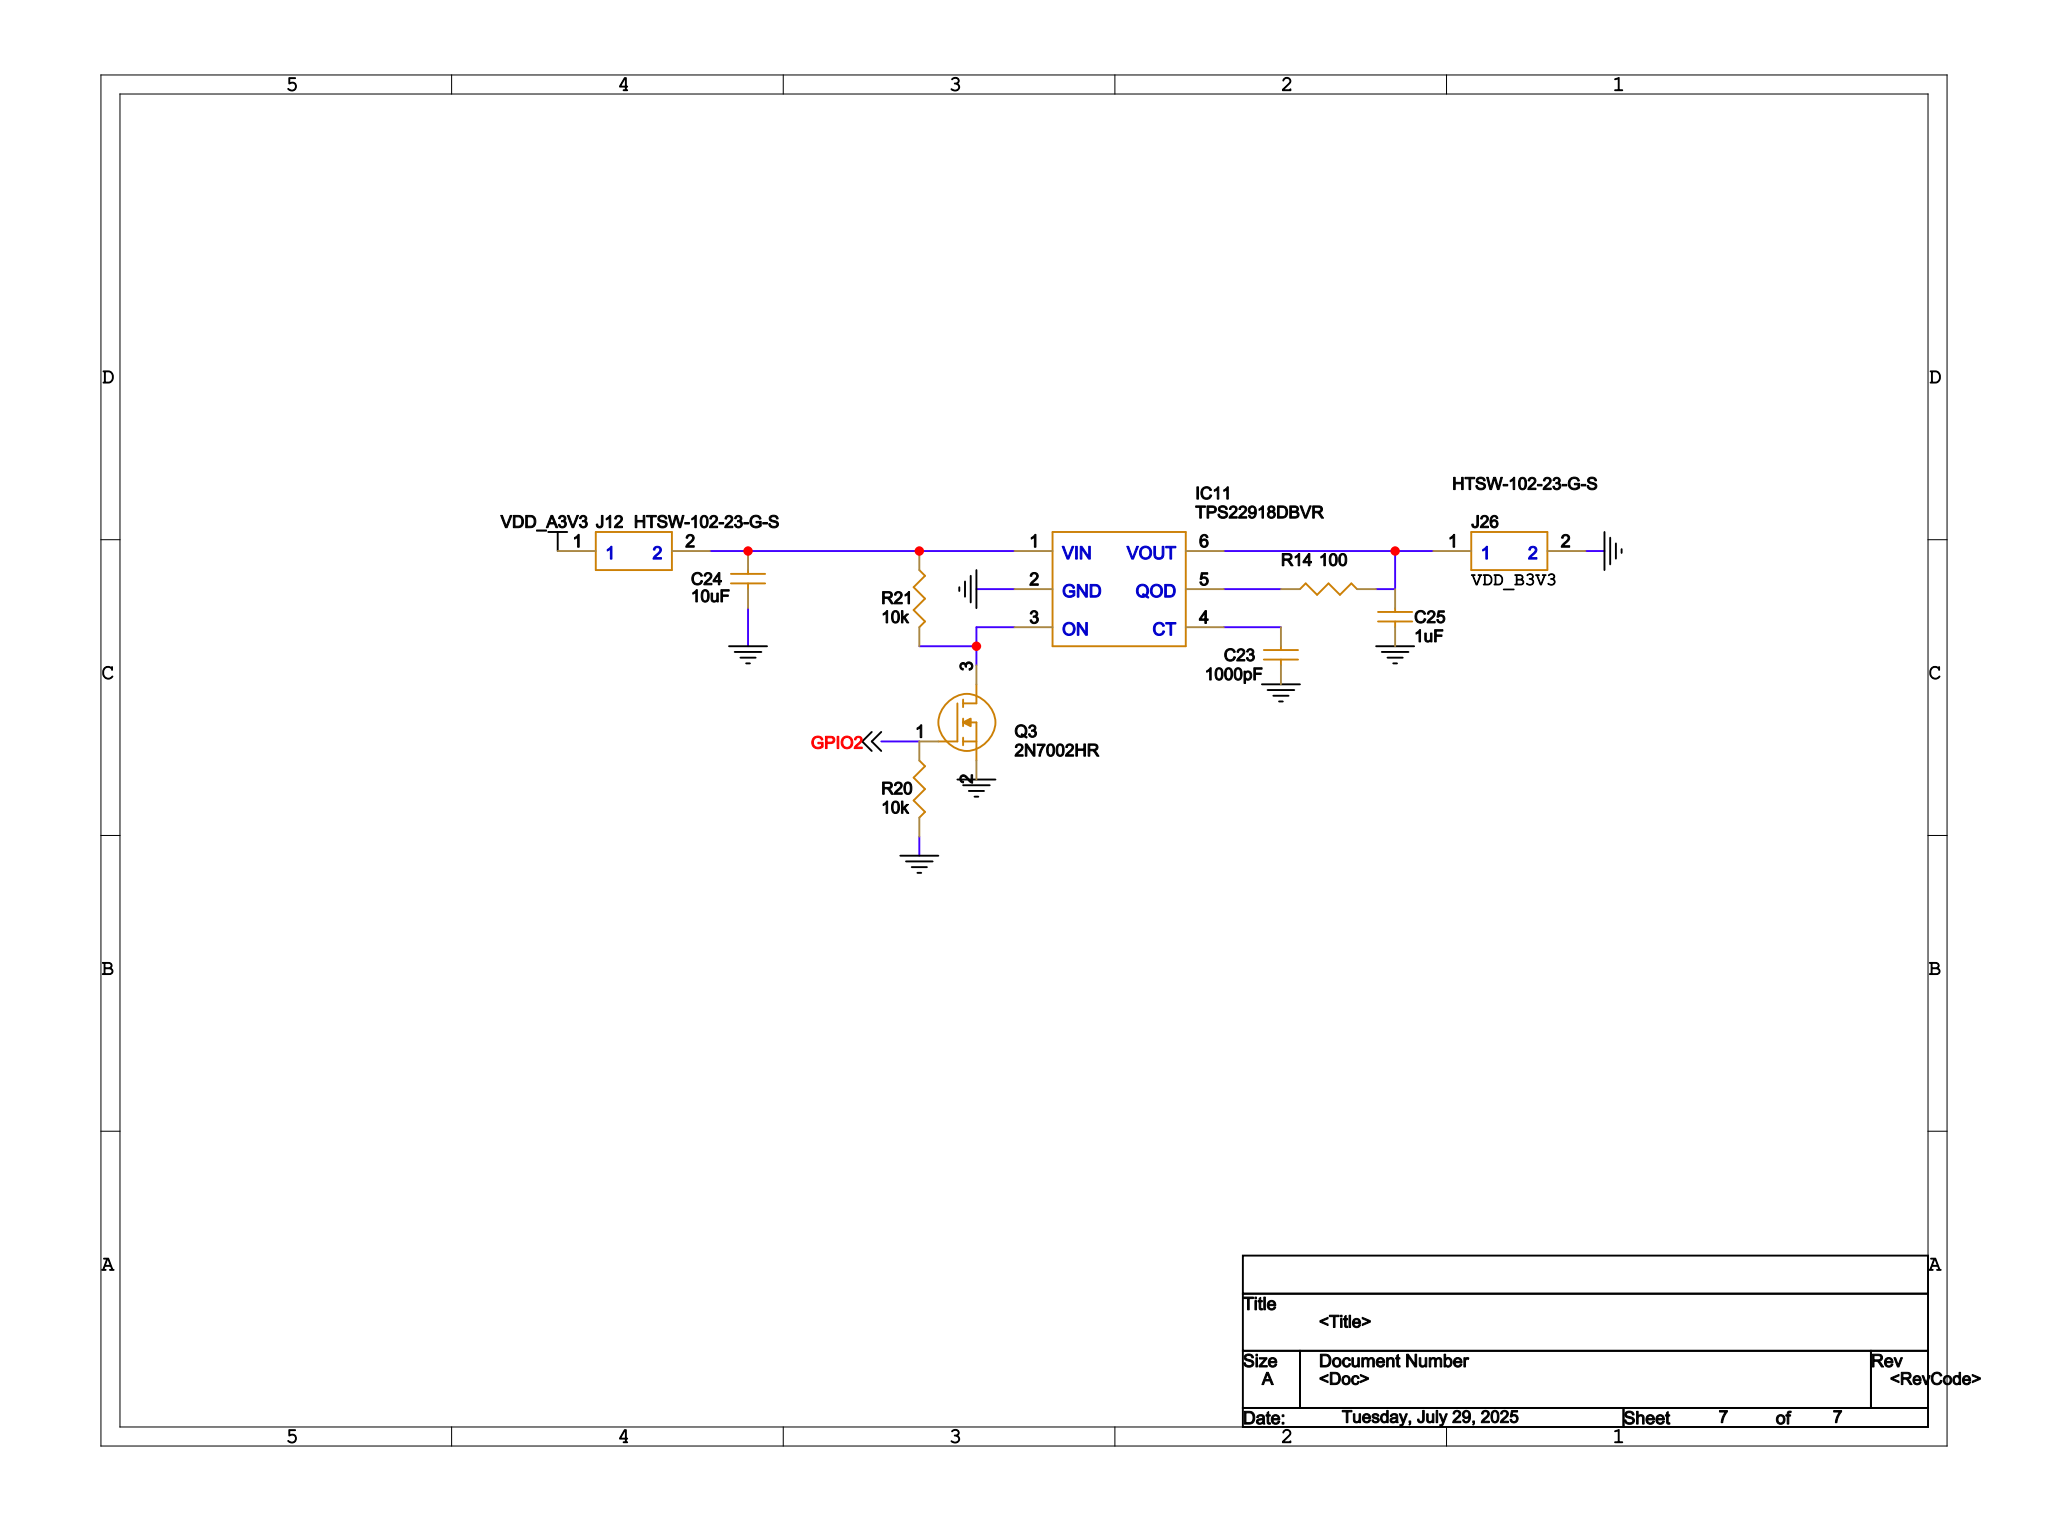Circuit board | Cadence Allegro | 93 parts | 49 nets | one sheet of the schematic
Parts on this sheet (reference | value | footprint):
C23 | 1000pF | C0402
C24 | 10uF | C1210
C25 | 1uF | C0402
IC11 | TPS22918DBVR | SOT95P280X145-6N
J12 | HTSW-102-23-G-S | HDRV2W64P0X254_1X2_508X248X838P
J26 | HTSW-102-23-G-S | HDRV2W64P0X254_1X2_508X248X838P
Q3 | 2N7002HR | SOT95P230X110-3N
R14 | 100 | R0402
R20 | 10k | R0402
R21 | 10k | R0402
Nets of these parts (net: part-pin ...):
GND: C23-2 C24-2 C25-2 IC11-2 J26-2 Q3-2 R20-2
VDD_A3V3: J12-1
N09097: C24-1 IC11-1 J12-2 R21-1
GPIO2: Q3-1 R20-1
N09150: C23-1 IC11-4
N09383: C25-1 IC11-6 J26-1 R14-2
N20640: IC11-3 Q3-3 R21-2
N09371: IC11-5 R14-1